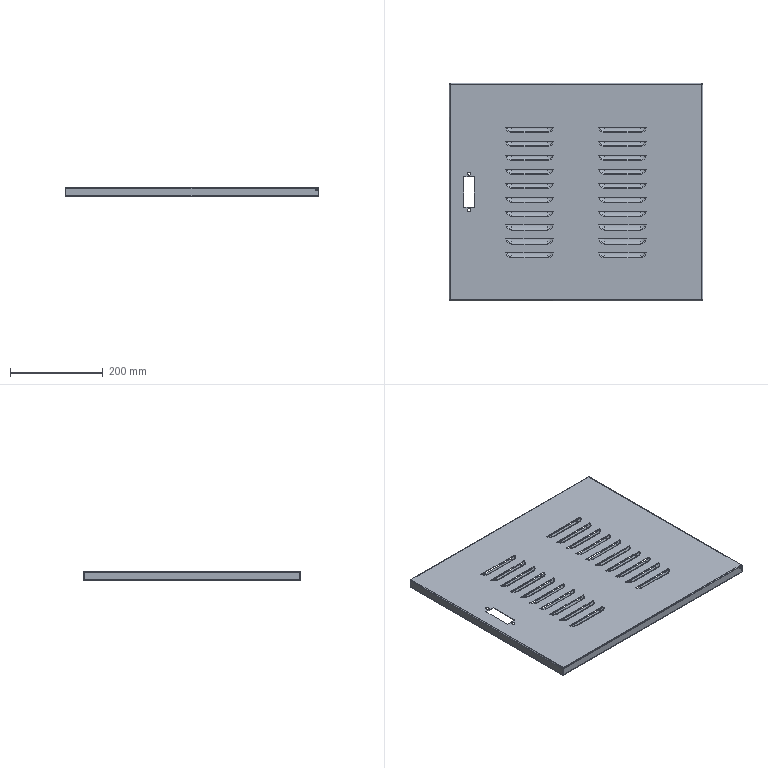Part | SolidWorks | features EdgeFlange 2, Cut 1, FlatPattern 1, FormToolInstance 1, ICE 1, SMBaseFlange 1, SheetMetal 1 | 1 solid | 442 faces | box 546 x 468 x 20 mm | volume 392970 mm3 | torus 160 | cylinder 104 | spline 96 | plane 82 | commonest cylinder face diameters 3.6 x20 6 x20 29 x20 31.4 x20 2 x8 4.4 x8